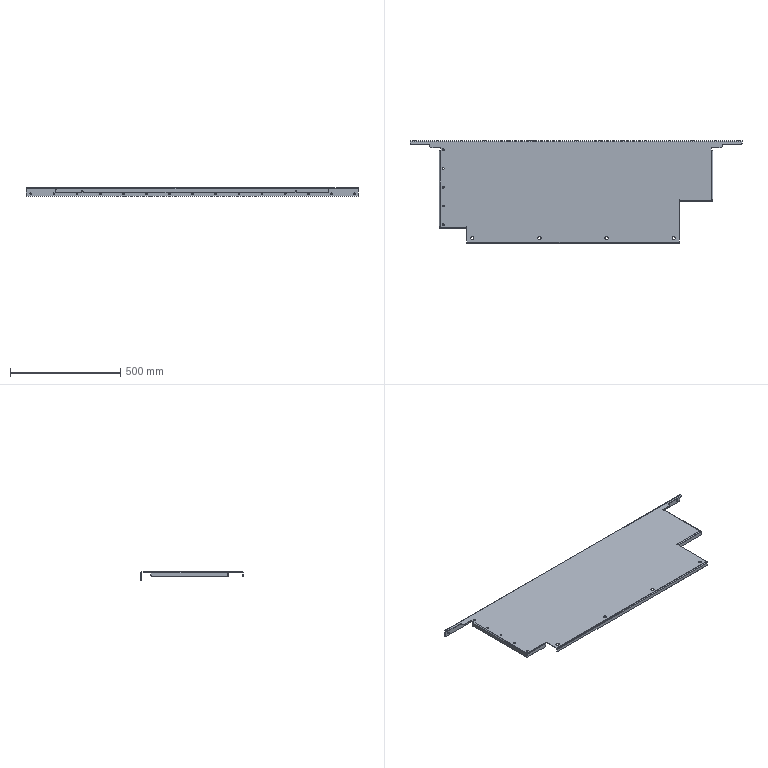Part | SolidWorks | features EdgeFlange 2, CornerRelief 1, Fillet 1, FlatPattern 1, ICE 1, SMBaseFlange 1, SheetMetal 1 | 1 solid | 144 faces | box 1508 x 463.5 x 37 mm | volume 1245074 mm3 | cylinder 84 | plane 56 | spline 4 | commonest cylinder face diameters 8 x46 10 x14 15 x8 5 x6 9 x6 4 x4